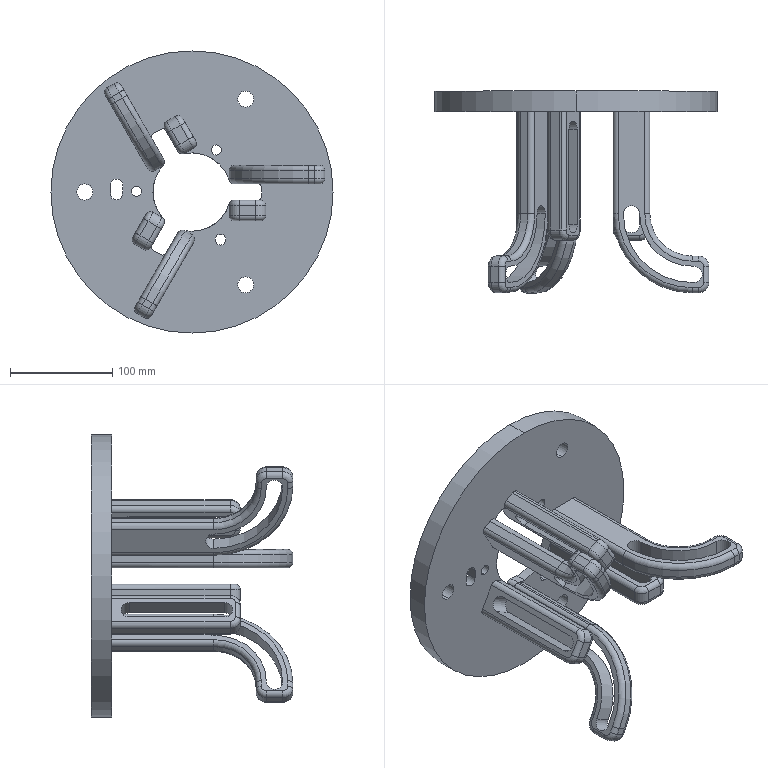Part | SolidWorks | features ICE 11, CirPattern 4, Cut 2, Fillet 2, Extrusion 1 | 1 solid | 215 faces | box 276 x 197.346 x 276 mm | volume 1375608 mm3 | cylinder 125 | plane 54 | torus 36 | commonest cylinder face diameters 10 x55 16 x12 20 x12 8 x7 15.75 x6 10.104 x4